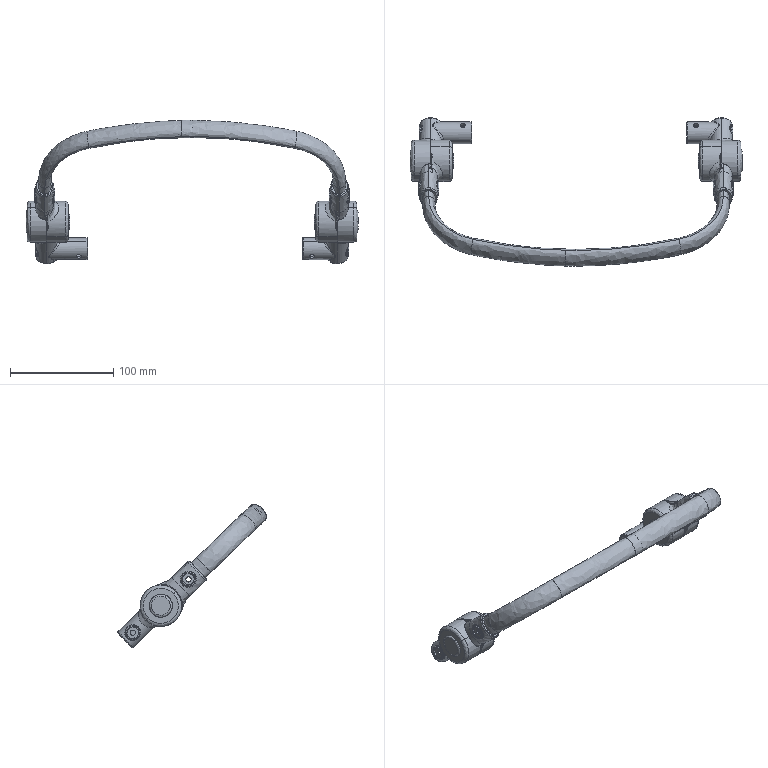Part | SolidWorks | 9 solids | 1223 faces | box 321.08 x 143.863 x 138.826 mm | volume 126881 mm3 | spline 635 | cylinder 335 | plane 228 | cone 14 | torus 11 | commonest cylinder face diameters 1.003 x58 5.2 x32 1 x30 34.6 x26 11 x16 14 x16